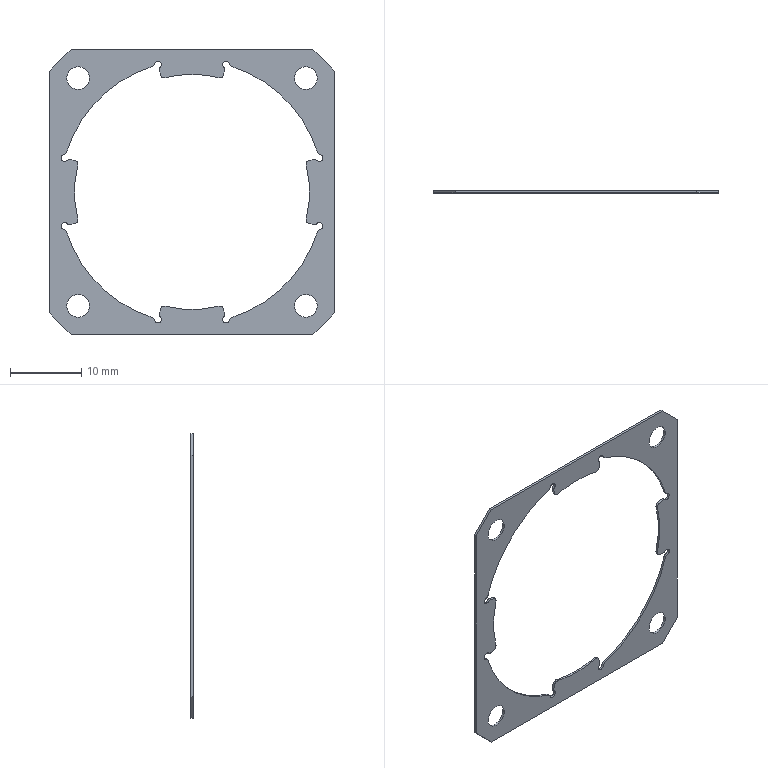Part | SolidWorks | features ICE 3, Extrusion 1, Fillet 1 | 1 solid | 75 faces | box 40 x 0.3 x 40 mm | volume 162.744 mm3 | cylinder 57 | plane 18 | commonest cylinder face diameters 1 x40 3.2 x8 33 x5 37 x4